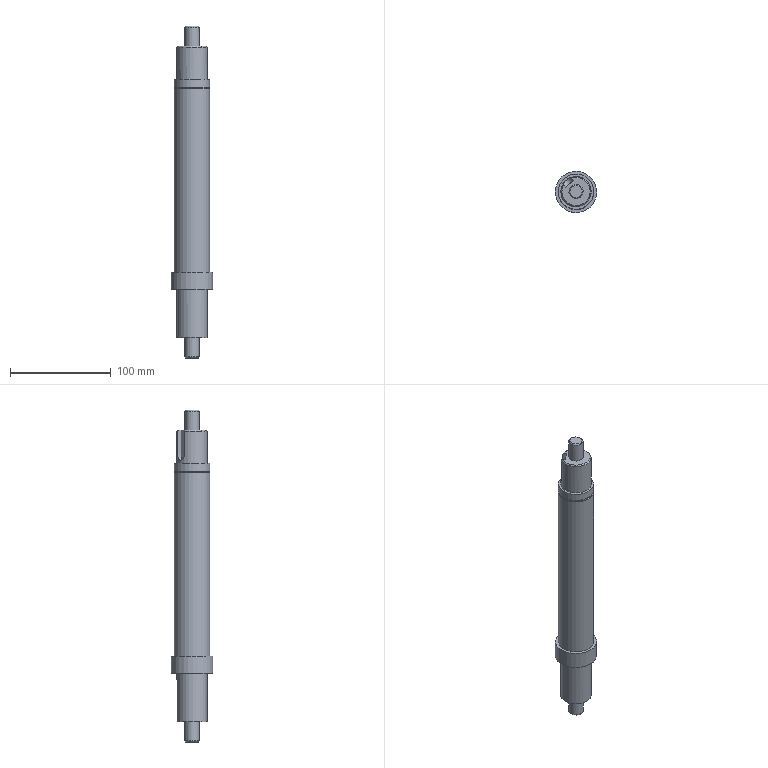Part | STEP file | HL4GZ-1.313.201 (left steering shaft) | 1 solid | 28 faces | box 41 x 41 x 329 mm | volume 265914 mm3 | plane 15 | cylinder 10 | cone 3 | commonest cylinder face diameters 10 x2 14 x2 30 x2 35 x2 33 x1 41 x1